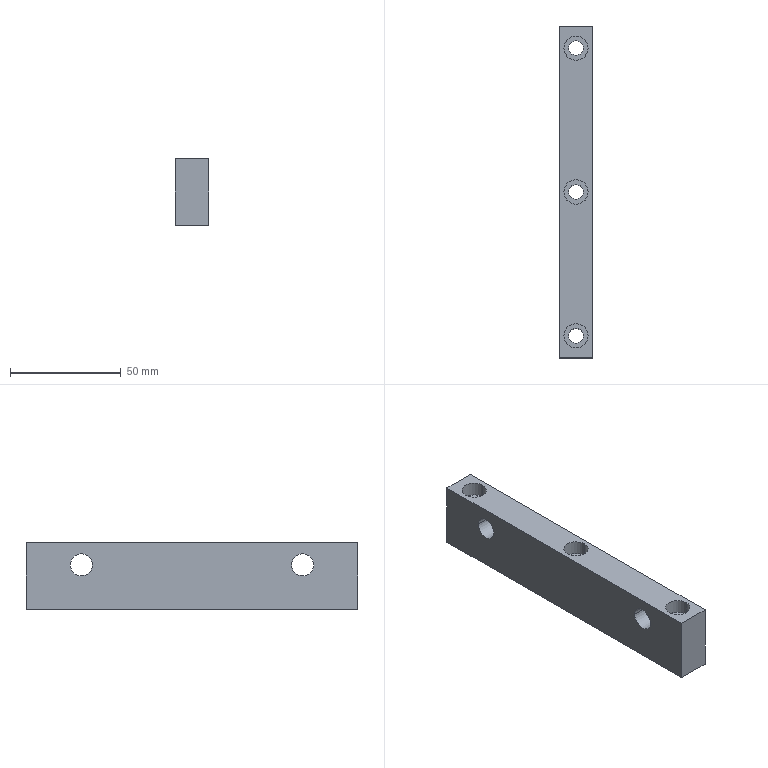Part | STEP file | ADJUT.BLOCK.stp | 1 solid | 25 faces | box 15 x 150 x 30 mm | volume 60879 mm3 | cylinder 10 | spline 8 | plane 7 | commonest cylinder face diameters 6.6 x4 11 x4 10 x2